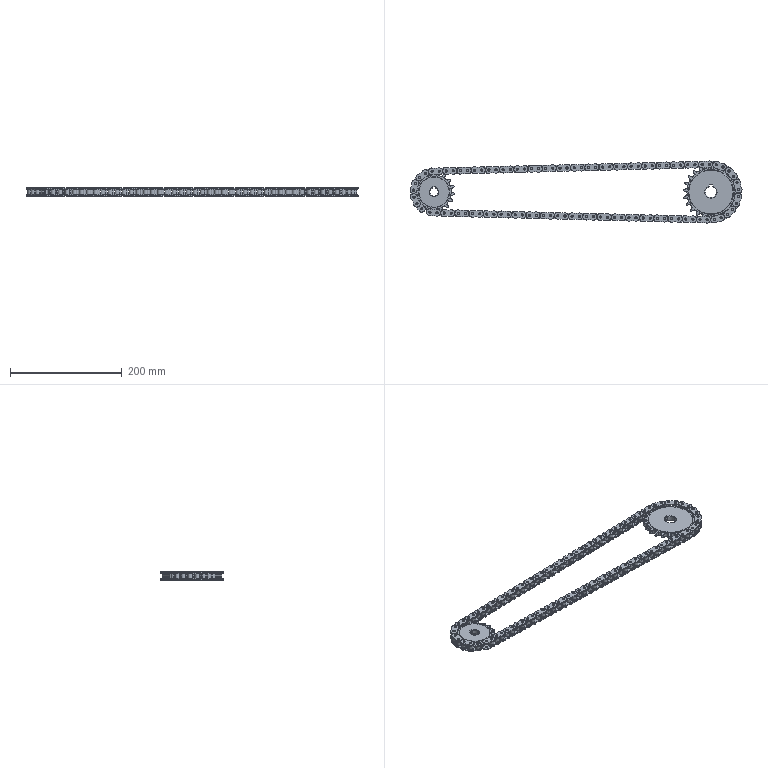Part | SolidWorks | features ReferencePattern 96, Belt 1, LocalChainPattern 1 | 149 solids | 3411 faces | volume 206432 mm3 | cylinder 2233 | plane 682 | cone 404 | torus 92 | commonest cylinder face diameters 3.98 x784 12.07 x294 12.33 x294 7.92 x196 43.376 x196 55.348 x196